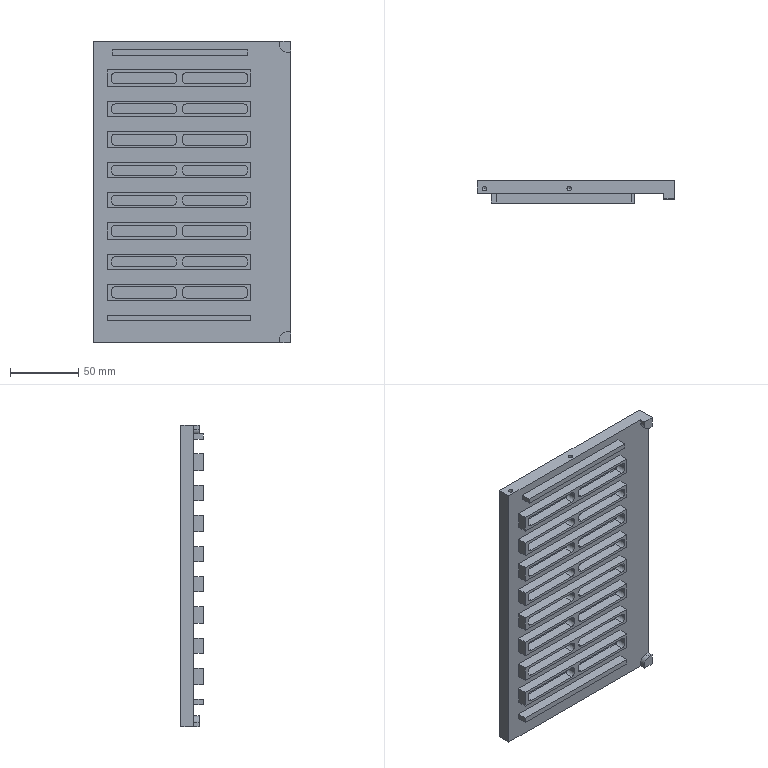NC program | NX | posted with a generic post | part box 144.5 x 16.5 x 221 mm
Lines 114 to 1205 of 11164:
(CAVITY_MILL , TOOL : D8-25-D8-60-3T-ROUGH)
N220 T02 M6
N222 G54
N224 G17 G0 G90 X4. Y-80.249 B0. C0. S4500 M3
N226 G43 Z20. H2
N228 Z2.533 B-180. C-180.
N230 G94 G1 Z-0.467 F3000.
N232 Y-76.649
N234 G3 X0. Y-72.649 R4.
N236 G1 X-110.527
N238 G2 X-110.898 Y-72.279 R0.4
N240 G1 Y72.279
N242 G2 X-110.527 Y72.649 R0.4
N244 G1 X-83.447
N246 Y66.249
N248 G3 X-85.1 Y63.183 R5.48
N250 X-86.753 Y66.249 R5.48
N252 G1 X-83.447
N254 X-79.732 Y67.73
N256 X-67.468
N258 G2 X-66.953 Y68.649 R4.
N260 G1 X-80.247
N262 G2 X-79.732 Y67.73 R4.
N264 G1 X-83.447 Y66.249
N266 Y72.649
N268 X-60.447
N270 Y66.249
N272 G3 X-62.1 Y63.183 R5.48
N274 X-63.753 Y66.249 R5.48
N276 G1 X-60.447
N278 X-56.732 Y67.73
N280 X-45.468
N282 G2 X-44.953 Y68.649 R4.
N284 G1 X-57.247
N286 G2 X-56.732 Y67.73 R4.
N288 G1 X-60.447 Y66.249
N290 Y72.649
N292 X-38.447
N294 Y66.249
N296 G3 X-40.1 Y63.183 R5.48
N298 X-41.753 Y66.249 R5.48
N300 G1 X-38.447
N302 X-34.732 Y67.73
N304 X-22.468
N306 G2 X-21.953 Y68.649 R4.
N308 G1 X-35.247
N310 G2 X-34.732 Y67.73 R4.
N312 G1 X-38.447 Y66.249
N314 Y72.649
N316 X-15.447
N318 Y66.249
N320 G3 X-17.1 Y63.183 R5.48
N322 X-18.753 Y66.249 R5.48
N324 G1 X-15.447
N326 X-11.732 Y67.73
N328 X-0.468
N330 G2 X0.047 Y68.649 R4.
N332 G1 X-12.247
N334 G2 X-11.732 Y67.73 R4.
N336 G1 X-15.447 Y66.249
N338 Y72.649
N340 X6.553
N342 Y66.249
N344 G3 X4.9 Y63.183 R5.48
N346 X3.247 Y66.249 R5.48
N348 G1 X6.553
N350 X10.268 Y67.73
N352 X21.532
N354 G2 X22.047 Y68.649 R4.
N356 G1 X9.753
N358 G2 X10.268 Y67.73 R4.
N360 G1 X6.553 Y66.249
N362 Y72.649
N364 X28.553
N366 Y66.249
N368 G3 X26.9 Y63.183 R5.48
N370 X25.247 Y66.249 R5.48
N372 G1 X28.553
N374 X32.268 Y67.73
N376 X44.532
N378 G2 X45.047 Y68.649 R4.
N380 G1 X31.753
N382 G2 X32.268 Y67.73 R4.
N384 G1 X28.553 Y66.249
N386 Y72.649
N388 X51.553
N390 Y66.249
N392 G3 X49.9 Y63.186 R5.48
N394 X48.247 Y66.249 R5.48
N396 G1 X51.553
N398 X55.268 Y67.73
N400 X66.532
N402 G2 X67.047 Y68.649 R4.
N404 G1 X54.753
N406 G2 X55.268 Y67.73 R4.
N408 G1 X51.553 Y66.249
N410 Y72.649
N412 X73.553
N414 Y66.249
N416 G3 X71.9 Y63.183 R5.48
N418 X70.247 Y66.249 R5.48
N420 G1 X73.553
N422 X77.268 Y67.73
N424 X89.532
N426 G2 X90.047 Y68.649 R4.
N428 G1 X76.753
N430 G2 X77.268 Y67.73 R4.
N432 G1 X73.553 Y66.249
N434 Y72.649
N436 X110.527
N438 G2 X110.898 Y72.279 R0.4
N440 G1 Y63.715
N442 X104.498
N444 G3 X104.1 Y63.73 R5.48
N446 G1 X100.3
N448 G3 X94.98 Y59.565 R5.48
N450 G1 Y62.25
N452 G3 X93.247 Y66.249 R5.48
N454 G1 X104.498
N456 Y63.715
N458 X110.898
N460 Y-72.279
N462 G2 X110.527 Y-72.649 R0.4
N464 G1 X0.
N466 Y-66.249
N468 X-104.498
N470 Y66.249
N472 X-98.247
N474 X-92.5 Y68.207
N476 X-98.247 Y66.249
N478 G3 X-99.98 Y62.25 R5.48
N480 G1 Y-42.75
N482 G3 X-94.503 Y-48.23 R5.48
N484 G1 X-90.5
N486 G3 X-85.1 Y-43.683 R5.48
N488 G1 X-86.361 Y-43.465
N490 G2 X-90.5 Y-46.95 R4.2
N492 G1 X-94.5
N494 G2 X-98.7 Y-42.75 R4.2
N496 G1 Y62.25
N498 G2 X-94.5 Y66.45 R4.2
N500 G1 X-90.5
N502 G2 X-86.3 Y62.25 R4.2
N504 G1 Y-42.75
N506 G2 X-86.361 Y-43.465 R4.2
N508 G1 X-85.1 Y-43.683
N510 G3 X-79.7 Y-48.23 R5.48
N512 G1 X-67.5
N514 G3 X-62.1 Y-43.683 R5.48
N516 G1 X-63.361 Y-43.465
N518 G2 X-67.5 Y-46.95 R4.2
N520 G1 X-79.7
N522 G2 X-83.9 Y-42.7 R4.2
N524 G1 Y62.25
N526 G2 X-79.7 Y66.45 R4.2
N528 G1 X-67.5
N530 G2 X-63.3 Y62.25 R4.2
N532 G1 Y-42.75
N534 G2 X-63.361 Y-43.465 R4.2
N536 G1 X-62.1 Y-43.683
N538 G3 X-56.7 Y-48.23 R5.48
N540 G1 X-45.496
N542 G3 X-40.1 Y-43.683 R5.48
N544 G1 X-41.361 Y-43.465
N546 G2 X-45.553 Y-46.95 R4.2
N548 G1 X-56.7
N550 G2 X-60.9 Y-42.7 R4.2
N552 G1 Y62.25
N554 G2 X-56.7 Y66.45 R4.2
N556 G1 X-45.5
N558 G2 X-41.3 Y62.25 R4.2
N560 G1 Y-42.75
N562 G2 X-41.361 Y-43.465 R4.2
N564 G1 X-40.1 Y-43.683
N566 G3 X-34.703 Y-48.23 R5.48
N568 G1 X-22.5
N570 G3 X-17.1 Y-43.683 R5.48
N572 G1 X-18.361 Y-43.465
N574 G2 X-22.5 Y-46.95 R4.2
N576 G1 X-34.7
N578 G2 X-38.9 Y-42.75 R4.2
N580 G1 Y62.25
N582 G2 X-34.7 Y66.45 R4.2
N584 G1 X-22.5
N586 G2 X-18.3 Y62.25 R4.2
N588 G1 Y-42.75
N590 G2 X-18.361 Y-43.465 R4.2
N592 G1 X-17.1 Y-43.683
N594 G3 X-11.7 Y-48.23 R5.48
N596 G1 X-0.608
N598 G3 X0.532 Y-48.132 R5.486
N600 X4.9 Y-43.683 R5.48
N602 G1 X3.639 Y-43.465
N604 G2 X0.29 Y-46.875 R4.2
N606 X-0.595 Y-46.95 R4.206
N608 G1 X-11.7
N610 G2 X-15.9 Y-42.75 R4.2
N612 G1 Y62.25
N614 G2 X-11.7 Y66.45 R4.2
N616 G1 X-0.5
N618 G2 X3.7 Y62.25 R4.2
N620 G1 Y-42.75
N622 G2 X3.639 Y-43.465 R4.2
N624 G1 X4.9 Y-43.683
N626 G3 X10.298 Y-48.23 R5.48
N628 G1 X21.5
N630 G3 X26.9 Y-43.683 R5.48
N632 G1 X25.639 Y-43.465
N634 G2 X21.5 Y-46.95 R4.2
N636 G1 X10.3
N638 G2 X6.1 Y-42.75 R4.2
N640 G1 Y62.25
N642 G2 X10.3 Y66.45 R4.2
N644 G1 X21.5
N646 G2 X25.7 Y62.25 R4.2
N648 G1 Y-42.75
N650 G2 X25.639 Y-43.465 R4.2
N652 G1 X26.9 Y-43.683
N654 G3 X32.3 Y-48.23 R5.48
N656 G1 X44.5
N658 G3 X49.9 Y-43.683 R5.48
N660 G1 X48.639 Y-43.465
N662 G2 X44.5 Y-46.95 R4.2
N664 G1 X32.3
N666 G2 X28.1 Y-42.75 R4.2
N668 G1 Y62.25
N670 G2 X32.3 Y66.45 R4.2
N672 G1 X44.5
N674 G2 X48.7 Y62.25 R4.2
N676 G1 Y-42.75
N678 G2 X48.639 Y-43.465 R4.2
N680 G1 X49.9 Y-43.683
N682 G3 X55.3 Y-48.23 R5.48
N684 G1 X66.5
N686 G3 X71.9 Y-43.683 R5.48
N688 G1 X70.639 Y-43.465
N690 G2 X66.5 Y-46.95 R4.2
N692 G1 X55.3
N694 G2 X51.1 Y-42.75 R4.2
N696 G1 Y62.693
N698 G3 X51.163 Y62.978 R7.083
N700 G2 X55.308 Y66.45 R4.2
N702 G1 X66.5
N704 G2 X70.7 Y62.25 R4.2
N706 G1 Y-42.75
N708 G2 X70.639 Y-43.465 R4.2
N710 G1 X71.9 Y-43.683
N712 G3 X77.297 Y-48.23 R5.48
N714 G1 X89.5
N716 G3 X94.98 Y-42.75 R5.48
N718 G1 Y-42.065
N720 X93.7
N722 Y-42.75
N724 G2 X89.5 Y-46.95 R4.2
N726 G1 X77.3
N728 G2 X73.1 Y-42.75 R4.2
N730 G1 Y62.25
N732 G2 X77.3 Y66.45 R4.2
N734 G1 X89.5
N736 G2 X93.7 Y62.25 R4.2
N738 G1 Y-42.065
N740 X94.98
N742 G3 X100.3 Y-46.23 R5.48
N744 G1 X104.1
N746 G3 X104.498 Y-46.215 R5.48
N748 G1 X104.405 Y-44.939
N750 G2 X104.1 Y-44.95 R4.2
N752 G1 X100.3
N754 G2 X96.1 Y-40.75 R4.2
N756 G1 Y58.25
N758 G2 X100.3 Y62.45 R4.2
N760 G1 X104.1
N762 G2 X108.3 Y58.25 R4.2
N764 G1 Y-40.75
N766 G2 X104.405 Y-44.939 R4.2
N768 G1 X104.498 Y-46.215
N770 Y-66.249
N772 X0.
N774 Y-59.849
N776 X-98.098
N778 Y-54.072
N780 X-100.314 Y-50.491
N782 X-98.098 Y-54.072
N784 G3 X-94.506 Y-54.63 R11.88
N786 G1 X-90.5
N788 G3 X-85.1 Y-53.332 R11.88
N790 X-79.7 Y-54.63 R11.88
N792 G1 X-67.5
N794 G3 X-62.1 Y-53.332 R11.88
N796 X-56.7 Y-54.63 R11.88
N798 G1 X-45.491
N800 G3 X-40.1 Y-53.332 R11.88
N802 X-34.706 Y-54.63 R11.88
N804 G1 X-22.5
N806 G3 X-17.1 Y-53.332 R11.88
N808 X-11.7 Y-54.63 R11.88
N810 G1 X-0.657
N812 G3 X1.74 Y-54.417 R11.886
N814 X4.9 Y-53.332 R11.88
N816 X10.295 Y-54.63 R11.88
N818 G1 X21.5
N820 G3 X26.9 Y-53.332 R11.88
N822 X32.3 Y-54.63 R11.88
N824 G1 X44.5
N826 G3 X49.9 Y-53.332 R11.88
N828 X55.3 Y-54.63 R11.88
N830 G1 X66.5
N832 G3 X71.9 Y-53.332 R11.88
N834 X77.292 Y-54.63 R11.88
N836 G1 X89.5
N838 G3 X96.818 Y-52.108 R11.88
N840 X98.098 Y-52.424 R11.88
N842 G1 Y-59.849
N844 X0.
N846 G3 X-4. Y-63.849 R4.
N848 G1 Y-80.249
N850 Z2.533
N852 G0 Z20.
N854 X4.
N856 Z2.067
N858 G1 Z-0.933
N860 Y-76.649
N862 G3 X0. Y-72.649 R4.
N864 G1 X-110.527
N866 G2 X-110.899 Y-72.279 R0.4
N868 G1 Y72.279
N870 G2 X-110.527 Y72.649 R0.4
N872 G1 X-83.447
N874 Y66.249
N876 G3 X-85.1 Y63.183 R5.48
N878 X-86.753 Y66.249 R5.48
N880 G1 X-83.447
N882 X-79.732 Y67.73
N884 X-67.468
N886 G2 X-66.953 Y68.649 R4.
N888 G1 X-80.247
N890 G2 X-79.732 Y67.73 R4.
N892 G1 X-83.447 Y66.249
N894 Y72.649
N896 X-60.447
N898 Y66.249
N900 G3 X-62.1 Y63.183 R5.48
N902 X-63.753 Y66.249 R5.48
N904 G1 X-60.447
N906 X-56.732 Y67.73
N908 X-45.468
N910 G2 X-44.953 Y68.649 R4.
N912 G1 X-57.247
N914 G2 X-56.732 Y67.73 R4.
N916 G1 X-60.447 Y66.249
N918 Y72.649
N920 X-38.447
N922 Y66.249
N924 G3 X-40.1 Y63.183 R5.48
N926 X-41.753 Y66.249 R5.48
N928 G1 X-38.447
N930 X-34.732 Y67.73
N932 X-22.468
N934 G2 X-21.953 Y68.649 R4.
N936 G1 X-35.247
N938 G2 X-34.732 Y67.73 R4.
N940 G1 X-38.447 Y66.249
N942 Y72.649
N944 X-15.447
N946 Y66.249
N948 G3 X-17.1 Y63.183 R5.48
N950 X-18.753 Y66.249 R5.48
N952 G1 X-15.447
N954 X-11.732 Y67.73
N956 X-0.468
N958 G2 X0.047 Y68.649 R4.
N960 G1 X-12.247
N962 G2 X-11.732 Y67.73 R4.
N964 G1 X-15.447 Y66.249
N966 Y72.649
N968 X6.553
N970 Y66.249
N972 G3 X4.9 Y63.183 R5.48
N974 X3.247 Y66.249 R5.48
N976 G1 X6.553
N978 X10.268 Y67.73
N980 X21.532
N982 G2 X22.047 Y68.649 R4.
N984 G1 X9.753
N986 G2 X10.268 Y67.73 R4.
N988 G1 X6.553 Y66.249
N990 Y72.649
N992 X28.553
N994 Y66.249
N996 G3 X26.9 Y63.183 R5.48
N998 X25.247 Y66.249 R5.48
N1000 G1 X28.553
N1002 X32.268 Y67.73
N1004 X44.532
N1006 G2 X45.047 Y68.649 R4.
N1008 G1 X31.753
N1010 G2 X32.268 Y67.73 R4.
N1012 G1 X28.553 Y66.249
N1014 Y72.649
N1016 X51.553
N1018 Y66.249
N1020 G3 X49.9 Y63.186 R5.48
N1022 X48.247 Y66.249 R5.48
N1024 G1 X51.553
N1026 X55.268 Y67.73
N1028 X66.532
N1030 G2 X67.047 Y68.649 R4.
N1032 G1 X54.753
N1034 G2 X55.268 Y67.73 R4.
N1036 G1 X51.553 Y66.249
N1038 Y72.649
N1040 X73.553
N1042 Y66.249
N1044 G3 X71.9 Y63.183 R5.48
N1046 X70.247 Y66.249 R5.48
N1048 G1 X73.553
N1050 X77.268 Y67.73
N1052 X89.532
N1054 G2 X90.047 Y68.649 R4.
N1056 G1 X76.753
N1058 G2 X77.268 Y67.73 R4.
N1060 G1 X73.553 Y66.249
N1062 Y72.649
N1064 X110.527
N1066 G2 X110.899 Y72.279 R0.4
N1068 G1 Y63.715
N1070 X104.499
N1072 G3 X104.1 Y63.73 R5.48
N1074 G1 X100.3
N1076 G3 X94.98 Y59.565 R5.48
N1078 G1 Y62.25
N1080 G3 X93.247 Y66.249 R5.48
N1082 G1 X104.499
N1084 Y63.715
N1086 X110.899
N1088 Y-72.279
N1090 G2 X110.527 Y-72.649 R0.4
N1092 G1 X0.
N1094 Y-66.249
N1096 X-104.499
N1098 Y66.249
N1100 X-98.247
N1102 X-92.5 Y68.207
N1104 X-98.247 Y66.249
N1106 G3 X-99.98 Y62.25 R5.48
N1108 G1 Y-42.75
N1110 G3 X-94.503 Y-48.23 R5.48
N1112 G1 X-90.5
N1114 G3 X-85.1 Y-43.683 R5.48
N1116 G1 X-86.361 Y-43.465
N1118 G2 X-90.5 Y-46.95 R4.2
N1120 G1 X-94.5
N1122 G2 X-98.7 Y-42.75 R4.2
N1124 G1 Y62.25
N1126 G2 X-94.5 Y66.45 R4.2
N1128 G1 X-90.5
N1130 G2 X-86.3 Y62.25 R4.2
N1132 G1 Y-42.75
N1134 G2 X-86.361 Y-43.465 R4.2
N1136 G1 X-85.1 Y-43.683
N1138 G3 X-79.7 Y-48.23 R5.48
N1140 G1 X-67.5
N1142 G3 X-62.1 Y-43.683 R5.48
N1144 G1 X-63.361 Y-43.465
N1146 G2 X-67.5 Y-46.95 R4.2
N1148 G1 X-79.7
N1150 G2 X-83.9 Y-42.7 R4.2
N1152 G1 Y62.25
N1154 G2 X-79.7 Y66.45 R4.2
N1156 G1 X-67.5
N1158 G2 X-63.3 Y62.25 R4.2
N1160 G1 Y-42.75
N1162 G2 X-63.361 Y-43.465 R4.2
N1164 G1 X-62.1 Y-43.683
N1166 G3 X-56.7 Y-48.23 R5.48
N1168 G1 X-45.496
N1170 G3 X-40.1 Y-43.683 R5.48
N1172 G1 X-41.361 Y-43.465
N1174 G2 X-43.779 Y-46.581 R4.2
N1176 X-45.553 Y-46.95 R4.2
N1178 G1 X-56.7
N1180 G2 X-60.9 Y-42.7 R4.2
N1182 G1 Y62.25
N1184 G2 X-56.7 Y66.45 R4.2
N1186 G1 X-45.5
N1188 G2 X-41.3 Y62.25 R4.2
N1190 G1 Y-42.75
N1192 G2 X-41.361 Y-43.465 R4.2
N1194 G1 X-40.1 Y-43.683
N1196 G3 X-34.703 Y-48.23 R5.48
N1198 G1 X-22.5
N1200 G3 X-17.1 Y-43.683 R5.48
N1202 G1 X-18.361 Y-43.465
N1204 G2 X-22.5 Y-46.95 R4.2
N1206 G1 X-34.7
N1208 G2 X-38.9 Y-42.75 R4.2
N1210 G1 Y62.25
N1212 G2 X-34.7 Y66.45 R4.2
N1214 G1 X-22.5
N1216 G2 X-18.3 Y62.25 R4.2
N1218 G1 Y-42.75
N1220 G2 X-18.361 Y-43.465 R4.2
N1222 G1 X-17.1 Y-43.683
N1224 G3 X-11.7 Y-48.23 R5.48
N1226 G1 X-0.608
N1228 G3 X0.532 Y-48.132 R5.486
N1230 X4.9 Y-43.683 R5.48
N1232 G1 X3.639 Y-43.465
N1234 G2 X0.29 Y-46.875 R4.2
N1236 X-0.595 Y-46.95 R4.206
N1238 G1 X-11.7
N1240 G2 X-15.9 Y-42.75 R4.2
N1242 G1 Y62.25
N1244 G2 X-11.7 Y66.45 R4.2
N1246 G1 X-0.5
N1248 G2 X3.7 Y62.25 R4.2
N1250 G1 Y-42.75
N1252 G2 X3.639 Y-43.465 R4.2
N1254 G1 X4.9 Y-43.683
N1256 G3 X10.297 Y-48.23 R5.48
N1258 G1 X21.5
N1260 G3 X26.9 Y-43.683 R5.48
N1262 G1 X25.639 Y-43.465
N1264 G2 X21.5 Y-46.95 R4.2
N1266 G1 X10.3
N1268 G2 X6.1 Y-42.75 R4.2
N1270 G1 Y62.25
N1272 G2 X10.3 Y66.45 R4.2
N1274 G1 X21.5
N1276 G2 X25.7 Y62.25 R4.2
N1278 G1 Y-42.75
N1280 G2 X25.639 Y-43.465 R4.2
N1282 G1 X26.9 Y-43.683
N1284 G3 X32.3 Y-48.23 R5.48
N1286 G1 X44.5
N1288 G3 X49.9 Y-43.683 R5.48
N1290 G1 X48.639 Y-43.465
N1292 G2 X44.5 Y-46.95 R4.2
N1294 G1 X32.3
N1296 G2 X28.1 Y-42.75 R4.2
N1298 G1 Y62.25
N1300 G2 X32.3 Y66.45 R4.2
N1302 G1 X44.5
N1304 G2 X48.7 Y62.25 R4.2
N1306 G1 Y-42.75
N1308 G2 X48.639 Y-43.465 R4.2
N1310 G1 X49.9 Y-43.683
N1312 G3 X55.3 Y-48.23 R5.48
N1314 G1 X66.5
N1316 G3 X71.9 Y-43.683 R5.48
N1318 G1 X70.639 Y-43.465
N1320 G2 X66.5 Y-46.95 R4.2
N1322 G1 X55.3
N1324 G2 X51.1 Y-42.75 R4.2
N1326 G1 Y62.693
N1328 G3 X51.163 Y62.978 R7.083
N1330 G2 X55.308 Y66.45 R4.2
N1332 G1 X66.5
N1334 G2 X70.7 Y62.25 R4.2
N1336 G1 Y-42.75
N1338 G2 X70.639 Y-43.465 R4.2
N1340 G1 X71.9 Y-43.683
N1342 G3 X77.297 Y-48.23 R5.48
N1344 G1 X89.502
N1346 G3 X94.98 Y-42.75 R5.48
N1348 G1 Y-42.065
N1350 X93.7
N1352 Y-42.75
N1354 G2 X89.5 Y-46.95 R4.2
N1356 G1 X77.3
N1358 G2 X73.1 Y-42.75 R4.2
N1360 G1 Y62.25
N1362 G2 X77.3 Y66.45 R4.2
N1364 G1 X89.5
N1366 G2 X93.7 Y62.25 R4.2
N1368 G1 Y-42.065
N1370 X94.98
N1372 G3 X100.3 Y-46.23 R5.48
N1374 G1 X104.1
N1376 G3 X104.499 Y-46.215 R5.48
N1378 G1 X104.405 Y-44.939
N1380 G2 X104.1 Y-44.95 R4.2
N1382 G1 X100.3
N1384 G2 X96.1 Y-40.75 R4.2
N1386 G1 Y58.25
N1388 G2 X100.3 Y62.45 R4.2
N1390 G1 X104.1
N1392 G2 X108.3 Y58.25 R4.2
N1394 G1 Y-40.75
N1396 G2 X104.405 Y-44.939 R4.2
N1398 G1 X104.499 Y-46.215
N1400 Y-66.249
N1402 X0.
N1404 Y-59.849
N1406 X-98.099
N1408 Y-54.072
N1410 X-100.314 Y-50.491
N1412 X-98.099 Y-54.072
N1414 G3 X-94.506 Y-54.63 R11.88
N1416 G1 X-90.5
N1418 G3 X-85.1 Y-53.332 R11.88
N1420 X-79.7 Y-54.63 R11.88
N1422 G1 X-67.5
N1424 G3 X-62.1 Y-53.332 R11.88
N1426 X-56.7 Y-54.63 R11.88
N1428 G1 X-45.491
N1430 G3 X-40.1 Y-53.332 R11.88
N1432 X-34.706 Y-54.63 R11.88
N1434 G1 X-22.5
N1436 G3 X-17.1 Y-53.332 R11.88
N1438 X-11.7 Y-54.63 R11.88
N1440 G1 X-0.657
N1442 G3 X1.74 Y-54.417 R11.886
N1444 X4.9 Y-53.332 R11.88
N1446 X10.295 Y-54.63 R11.88
N1448 G1 X21.5
N1450 G3 X26.9 Y-53.332 R11.88
N1452 X32.3 Y-54.63 R11.88
N1454 G1 X44.5
N1456 G3 X49.9 Y-53.332 R11.88
N1458 X55.3 Y-54.63 R11.88
N1460 G1 X66.5
N1462 G3 X71.9 Y-53.332 R11.88
N1464 X77.292 Y-54.63 R11.88
N1466 G1 X89.504
N1468 G3 X96.818 Y-52.108 R11.88
N1470 X98.099 Y-52.424 R11.88
N1472 G1 Y-59.849
N1474 X0.
N1476 G3 X-4. Y-63.849 R4.
N1478 G1 Y-80.249
N1480 Z2.067
N1482 G0 Z20.
N1484 X4.
N1486 Z1.6
N1488 G1 Z-1.4
N1490 Y-76.649
N1492 G3 X0. Y-72.649 R4.
N1494 G1 X-110.527
N1496 G2 X-110.899 Y-72.279 R0.4
N1498 G1 Y72.279
N1500 G2 X-110.527 Y72.649 R0.4
N1502 G1 X-83.447
N1504 Y66.249
N1506 G3 X-85.1 Y63.183 R5.48
N1508 X-86.753 Y66.249 R5.48
N1510 G1 X-83.447
N1512 X-79.732 Y67.73
N1514 X-67.469
N1516 G2 X-66.953 Y68.649 R4.
N1518 G1 X-80.247
N1520 G2 X-79.732 Y67.73 R4.
N1522 G1 X-83.447 Y66.249
N1524 Y72.649
N1526 X-60.447
N1528 Y66.249
N1530 G3 X-62.1 Y63.183 R5.48
N1532 X-63.753 Y66.249 R5.48
N1534 G1 X-60.447
N1536 X-56.732 Y67.73
N1538 X-45.469
N1540 G2 X-44.953 Y68.649 R4.
N1542 G1 X-57.247
N1544 G2 X-56.732 Y67.73 R4.
N1546 G1 X-60.447 Y66.249
N1548 Y72.649
N1550 X-38.447
N1552 Y66.249
N1554 G3 X-40.1 Y63.183 R5.48
N1556 X-41.753 Y66.249 R5.48
N1558 G1 X-38.447
N1560 X-34.732 Y67.73
N1562 X-22.469
N1564 G2 X-21.953 Y68.649 R4.
N1566 G1 X-35.247
N1568 G2 X-34.732 Y67.73 R4.
N1570 G1 X-38.447 Y66.249
N1572 Y72.649
N1574 X-15.447
N1576 Y66.249
N1578 G3 X-17.1 Y63.183 R5.48
N1580 X-18.753 Y66.249 R5.48
N1582 G1 X-15.447
N1584 X-11.732 Y67.73
N1586 X-0.469
N1588 G2 X0.047 Y68.649 R4.
N1590 G1 X-12.247
N1592 G2 X-11.732 Y67.73 R4.
N1594 G1 X-15.447 Y66.249
N1596 Y72.649
N1598 X6.553
N1600 Y66.249
N1602 G3 X4.9 Y63.183 R5.48
N1604 X3.247 Y66.249 R5.48
N1606 G1 X6.553
N1608 X10.268 Y67.73
N1610 X21.531
N1612 G2 X22.047 Y68.649 R4.
N1614 G1 X9.753
N1616 G2 X10.268 Y67.73 R4.
N1618 G1 X6.553 Y66.249
N1620 Y72.649
N1622 X28.553
N1624 Y66.249
N1626 G3 X26.9 Y63.183 R5.48
N1628 X25.247 Y66.249 R5.48
N1630 G1 X28.553
N1632 X32.268 Y67.73
N1634 X44.531
N1636 G2 X45.047 Y68.649 R4.
N1638 G1 X31.753
N1640 G2 X32.268 Y67.73 R4.
N1642 G1 X28.553 Y66.249
N1644 Y72.649
N1646 X51.553
N1648 Y66.249
N1650 G3 X49.9 Y63.186 R5.48
N1652 X48.247 Y66.249 R5.48
N1654 G1 X51.553
N1656 X55.268 Y67.73
N1658 X66.531
N1660 G2 X67.047 Y68.649 R4.
N1662 G1 X54.753
N1664 G2 X55.268 Y67.73 R4.
N1666 G1 X51.553 Y66.249
N1668 Y72.649
N1670 X73.553
N1672 Y66.249
N1674 G3 X71.9 Y63.183 R5.48
N1676 X70.247 Y66.249 R5.48
N1678 G1 X73.553
N1680 X77.268 Y67.73
N1682 X89.531
N1684 G2 X90.047 Y68.649 R4.
N1686 G1 X76.753
N1688 G2 X77.268 Y67.73 R4.
N1690 G1 X73.553 Y66.249
N1692 Y72.649
N1694 X110.527
N1696 G2 X110.899 Y72.279 R0.4
N1698 G1 Y63.715
N1700 X104.499
N1702 G3 X104.1 Y63.73 R5.48
N1704 G1 X100.3
N1706 G3 X94.98 Y59.565 R5.48
N1708 G1 Y62.25
N1710 G3 X93.247 Y66.249 R5.48
N1712 G1 X104.499
N1714 Y63.715
N1716 X110.899
N1718 Y-72.279
N1720 G2 X110.527 Y-72.649 R0.4
N1722 G1 X0.
N1724 Y-66.249
N1726 X-104.499
N1728 Y66.249
N1730 X-98.247
N1732 X-92.5 Y68.207
N1734 X-98.247 Y66.249
N1736 G3 X-99.98 Y62.25 R5.48
N1738 G1 Y-42.75
N1740 G3 X-94.5 Y-48.23 R5.48
N1742 G1 X-90.5
N1744 G3 X-85.1 Y-43.683 R5.48
N1746 G1 X-86.361 Y-43.465
N1748 G2 X-90.5 Y-46.95 R4.2
N1750 G1 X-94.5
N1752 G2 X-98.7 Y-42.75 R4.2
N1754 G1 Y62.25
N1756 G2 X-94.5 Y66.45 R4.2
N1758 G1 X-90.5
N1760 G2 X-86.3 Y62.25 R4.2
N1762 G1 Y-42.75
N1764 G2 X-86.361 Y-43.465 R4.2
N1766 G1 X-85.1 Y-43.683
N1768 G3 X-79.7 Y-48.23 R5.48
N1770 G1 X-67.5
N1772 G3 X-62.1 Y-43.683 R5.48
N1774 G1 X-63.361 Y-43.465
N1776 G2 X-67.5 Y-46.95 R4.2
N1778 G1 X-79.7
N1780 G2 X-83.9 Y-42.75 R4.2
N1782 G1 Y62.25
N1784 G2 X-79.7 Y66.45 R4.2
N1786 G1 X-67.5
N1788 G2 X-63.3 Y62.25 R4.2
N1790 G1 Y-42.75
N1792 G2 X-63.361 Y-43.465 R4.2
N1794 G1 X-62.1 Y-43.683
N1796 G3 X-56.7 Y-48.23 R5.48
N1798 G1 X-45.5
N1800 G3 X-40.1 Y-43.683 R5.48
N1802 G1 X-41.361 Y-43.465
N1804 G2 X-45.552 Y-46.95 R4.2
N1806 G1 X-56.7
N1808 G2 X-60.9 Y-42.75 R4.2
N1810 G1 Y62.25
N1812 G2 X-56.7 Y66.45 R4.2
N1814 G1 X-45.5
N1816 G2 X-41.3 Y62.25 R4.2
N1818 G1 Y-42.75
N1820 G2 X-41.361 Y-43.465 R4.2
N1822 G1 X-40.1 Y-43.683
N1824 G3 X-34.7 Y-48.23 R5.48
N1826 G1 X-22.5
N1828 G3 X-17.1 Y-43.683 R5.48
N1830 G1 X-18.361 Y-43.465
N1832 G2 X-22.5 Y-46.95 R4.2
N1834 G1 X-34.7
N1836 G2 X-38.9 Y-42.75 R4.2
N1838 G1 Y62.25
N1840 G2 X-34.7 Y66.45 R4.2
N1842 G1 X-22.5
N1844 G2 X-18.3 Y62.25 R4.2
N1846 G1 Y-42.75
N1848 G2 X-18.361 Y-43.465 R4.2
N1850 G1 X-17.1 Y-43.683
N1852 G3 X-11.7 Y-48.23 R5.48
N1854 G1 X-0.608
N1856 G3 X0.532 Y-48.132 R5.486
N1858 X4.9 Y-43.683 R5.48
N1860 G1 X3.639 Y-43.465
N1862 G2 X0.29 Y-46.875 R4.2
N1864 X-0.595 Y-46.95 R4.206
N1866 G1 X-11.7
N1868 G2 X-15.9 Y-42.75 R4.2
N1870 G1 Y62.25
N1872 G2 X-11.7 Y66.45 R4.2
N1874 G1 X-0.5
N1876 G2 X3.7 Y62.25 R4.2
N1878 G1 Y-42.75
N1880 G2 X3.639 Y-43.465 R4.2
N1882 G1 X4.9 Y-43.683
N1884 G3 X10.3 Y-48.23 R5.48
N1886 G1 X21.5
N1888 G3 X26.9 Y-43.683 R5.48
N1890 G1 X25.639 Y-43.465
N1892 G2 X21.5 Y-46.95 R4.2
N1894 G1 X10.3
N1896 G2 X6.1 Y-42.75 R4.2
N1898 G1 Y62.25
N1900 G2 X10.3 Y66.45 R4.2
N1902 G1 X21.5
N1904 G2 X25.7 Y62.25 R4.2
N1906 G1 Y-42.75
N1908 G2 X25.639 Y-43.465 R4.2
N1910 G1 X26.9 Y-43.683
N1912 G3 X32.3 Y-48.23 R5.48
N1914 G1 X44.5
N1916 G3 X49.9 Y-43.683 R5.48
N1918 G1 X48.639 Y-43.465
N1920 G2 X44.5 Y-46.95 R4.2
N1922 G1 X32.3
N1924 G2 X28.1 Y-42.75 R4.2
N1926 G1 Y62.25
N1928 G2 X32.3 Y66.45 R4.2
N1930 G1 X44.5
N1932 G2 X48.7 Y62.25 R4.2
N1934 G1 Y-42.75
N1936 G2 X48.639 Y-43.465 R4.2
N1938 G1 X49.9 Y-43.683
N1940 G3 X55.3 Y-48.23 R5.48
N1942 G1 X66.5
N1944 G3 X71.9 Y-43.683 R5.48
N1946 G1 X70.639 Y-43.465
N1948 G2 X66.5 Y-46.95 R4.2
N1950 G1 X55.3
N1952 G2 X51.1 Y-42.75 R4.2
N1954 G1 Y62.693
N1956 G3 X51.163 Y62.978 R7.083
N1958 G2 X55.3 Y66.45 R4.2
N1960 G1 X66.5
N1962 G2 X70.7 Y62.25 R4.2
N1964 G1 Y-42.75
N1966 G2 X70.639 Y-43.465 R4.2
N1968 G1 X71.9 Y-43.683
N1970 G3 X77.3 Y-48.23 R5.48
N1972 G1 X89.5
N1974 G3 X94.98 Y-42.75 R5.48
N1976 G1 Y-42.065
N1978 X93.7
N1980 Y-42.75
N1982 G2 X89.5 Y-46.95 R4.2
N1984 G1 X77.3
N1986 G2 X73.1 Y-42.75 R4.2
N1988 G1 Y62.25
N1990 G2 X77.3 Y66.45 R4.2
N1992 G1 X89.5
N1994 G2 X93.7 Y62.25 R4.2
N1996 G1 Y-42.065
N1998 X94.98
N2000 G3 X100.3 Y-46.23 R5.48
N2002 G1 X104.1
N2004 G3 X104.499 Y-46.215 R5.48
N2006 G1 X104.405 Y-44.939
N2008 G2 X104.1 Y-44.95 R4.2
N2010 G1 X100.3
N2012 G2 X96.1 Y-40.75 R4.2
N2014 G1 Y58.25
N2016 G2 X100.3 Y62.45 R4.2
N2018 G1 X104.1
N2020 G2 X108.3 Y58.25 R4.2
N2022 G1 Y-40.75
N2024 G2 X104.405 Y-44.939 R4.2
N2026 G1 X104.499 Y-46.215
N2028 Y-66.249
N2030 X0.
N2032 Y-59.849
N2034 X-98.099
N2036 Y-54.072
N2038 X-100.314 Y-50.491
N2040 X-98.099 Y-54.072
N2042 G3 X-94.5 Y-54.63 R11.88
N2044 G1 X-90.5
N2046 G3 X-85.1 Y-53.332 R11.88
N2048 X-79.7 Y-54.63 R11.88
N2050 G1 X-67.5
N2052 G3 X-62.1 Y-53.332 R11.88
N2054 X-56.7 Y-54.63 R11.88
N2056 G1 X-45.5
N2058 G3 X-40.1 Y-53.332 R11.88
N2060 X-34.7 Y-54.63 R11.88
N2062 G1 X-22.5
N2064 G3 X-17.1 Y-53.332 R11.88
N2066 X-11.7 Y-54.63 R11.88
N2068 G1 X-0.657
N2070 G3 X1.739 Y-54.417 R11.886
N2072 X4.9 Y-53.332 R11.88
N2074 X10.3 Y-54.63 R11.88
N2076 G1 X21.5
N2078 G3 X26.9 Y-53.332 R11.88
N2080 X32.3 Y-54.63 R11.88
N2082 G1 X44.5
N2084 G3 X49.9 Y-53.332 R11.88
N2086 X55.3 Y-54.63 R11.88
N2088 G1 X66.5
N2090 G3 X71.9 Y-53.332 R11.88
N2092 X77.3 Y-54.63 R11.88
N2094 G1 X89.5
N2096 G3 X96.818 Y-52.108 R11.88
N2098 X98.099 Y-52.424 R11.88
N2100 G1 Y-59.849
N2102 X0.
N2104 G3 X-4. Y-63.849 R4.
N2106 G1 Y-80.249
N2108 Z1.6
N2110 G0 Z20.
N2112 X4.
N2114 Z1.133
N2116 G1 Z-1.867
N2118 Y-76.649
N2120 G3 X0. Y-72.649 R4.
N2122 G1 X-110.527
N2124 G2 X-110.899 Y-72.279 R0.4
N2126 G1 Y72.279
N2128 G2 X-110.527 Y72.649 R0.4
N2130 G1 X-83.447
N2132 Y66.249
N2134 G3 X-85.1 Y63.183 R5.48
N2136 X-86.753 Y66.249 R5.48
N2138 G1 X-83.447
N2140 X-79.731 Y67.73
N2142 X-67.469
N2144 G2 X-66.953 Y68.649 R4.
N2146 G1 X-80.247
N2148 G2 X-79.731 Y67.73 R4.
N2150 G1 X-83.447 Y66.249
N2152 Y72.649
N2154 X-60.447
N2156 Y66.249
N2158 G3 X-62.1 Y63.183 R5.48
N2160 X-63.753 Y66.249 R5.48
N2162 G1 X-60.447
N2164 X-56.731 Y67.73
N2166 X-45.469
N2168 G2 X-44.953 Y68.649 R4.
N2170 G1 X-57.247
N2172 G2 X-56.731 Y67.73 R4.
N2174 G1 X-60.447 Y66.249
N2176 Y72.649
N2178 X-38.447
N2180 Y66.249
N2182 G3 X-40.1 Y63.183 R5.48
N2184 X-41.753 Y66.249 R5.48
N2186 G1 X-38.447
N2188 X-34.731 Y67.73
N2190 X-22.469
N2192 G2 X-21.953 Y68.649 R4.
N2194 G1 X-35.247
N2196 G2 X-34.731 Y67.73 R4.
N2198 G1 X-38.447 Y66.249
N2200 Y72.649
N2202 X-15.447
N2204 Y66.249
N2206 G3 X-17.1 Y63.183 R5.48
N2208 X-18.753 Y66.249 R5.48
N2210 G1 X-15.447
N2212 X-11.731 Y67.73
N2214 X-0.469
N2216 G2 X0.047 Y68.649 R4.
N2218 G1 X-12.247
N2220 G2 X-11.731 Y67.73 R4.
N2222 G1 X-15.447 Y66.249
N2224 Y72.649
N2226 X6.553
N2228 Y66.249
N2230 G3 X4.9 Y63.183 R5.48
N2232 X3.247 Y66.249 R5.48
N2234 G1 X6.553
N2236 X10.269 Y67.73
N2238 X21.531
N2240 G2 X22.047 Y68.649 R4.
N2242 G1 X9.753
N2244 G2 X10.269 Y67.73 R4.
N2246 G1 X6.553 Y66.249
N2248 Y72.649
N2250 X28.553
N2252 Y66.249
N2254 G3 X26.9 Y63.183 R5.48
N2256 X25.247 Y66.249 R5.48
N2258 G1 X28.553
N2260 X32.269 Y67.73
N2262 X44.531
N2264 G2 X45.047 Y68.649 R4.
N2266 G1 X31.753
N2268 G2 X32.269 Y67.73 R4.
N2270 G1 X28.553 Y66.249
N2272 Y72.649
N2274 X51.553
N2276 Y66.249
N2278 G3 X49.9 Y63.186 R5.48
N2280 X48.247 Y66.249 R5.48
N2282 G1 X51.553
N2284 X55.269 Y67.73
N2286 X66.531
N2288 G2 X67.047 Y68.649 R4.
N2290 G1 X54.753
N2292 G2 X55.269 Y67.73 R4.
N2294 G1 X51.553 Y66.249
N2296 Y72.649
N2298 X73.553
N2300 Y66.249
N2302 G3 X71.9 Y63.183 R5.48
N2304 X70.247 Y66.249 R5.48
N2306 G1 X73.553
N2308 X77.269 Y67.73
N2310 X89.531
N2312 G2 X90.047 Y68.649 R4.
N2314 G1 X76.753
N2316 G2 X77.269 Y67.73 R4.
N2318 G1 X73.553 Y66.249
N2320 Y72.649
N2322 X110.527
N2324 G2 X110.899 Y72.279 R0.4
N2326 G1 Y63.715
N2328 X104.499
N2330 G3 X104.1 Y63.73 R5.48
N2332 G1 X100.3
N2334 G3 X94.98 Y59.565 R5.48
N2336 G1 Y62.25
N2338 G3 X93.247 Y66.249 R5.48
N2340 G1 X104.499
N2342 Y63.715
N2344 X110.899
N2346 Y-72.279
N2348 G2 X110.527 Y-72.649 R0.4
N2350 G1 X0.
N2352 Y-66.249
N2354 X-104.499
N2356 Y66.249
N2358 X-98.247
N2360 X-92.5 Y68.207
N2362 X-98.247 Y66.249
N2364 G3 X-99.98 Y62.25 R5.48
N2366 G1 Y-42.75
N2368 G3 X-94.5 Y-48.23 R5.48
N2370 G1 X-90.5
N2372 G3 X-85.1 Y-43.683 R5.48
N2374 G1 X-86.361 Y-43.465
N2376 G2 X-90.5 Y-46.95 R4.2
N2378 G1 X-94.5
N2380 G2 X-98.7 Y-42.75 R4.2
N2382 G1 Y62.25
N2384 G2 X-94.5 Y66.45 R4.2
N2386 G1 X-90.5
N2388 G2 X-86.3 Y62.25 R4.2
N2390 G1 Y-42.75
N2392 G2 X-86.361 Y-43.465 R4.2
N2394 G1 X-85.1 Y-43.683
N2396 G3 X-79.7 Y-48.23 R5.48